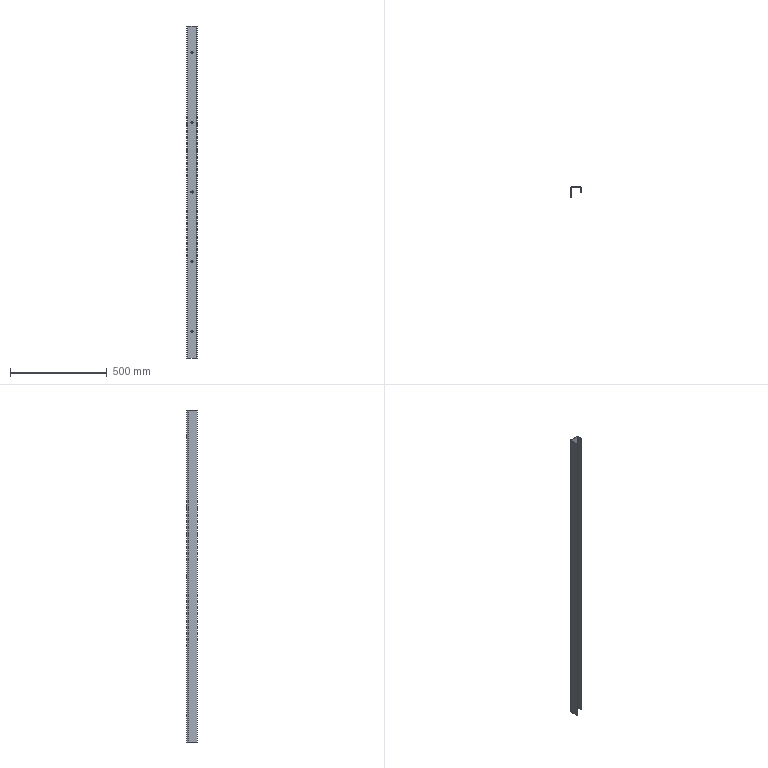Part | STEP file | SYL_0392D6J1SYL0380DJ10-1409429 | 1 solid | 32 faces | box 55 x 53 x 1714 mm | volume 657582 mm3 | plane 18 | cylinder 14 | commonest cylinder face diameters 10.5 x10 6 x2 12 x2
STEP:
#1=CARTESIAN_POINT('',(27.5,-3.,-725.25));
#2=VERTEX_POINT('',#1);
#3=CARTESIAN_POINT('',(27.5,0.,-725.25));
#4=VERTEX_POINT('',#3);
#5=CARTESIAN_POINT('',(27.5,0.,-725.25));
#6=DIRECTION('',(0.,1.,0.));
#7=VECTOR('',#6,1000.);
#8=LINE('',#5,#7);
#9=EDGE_CURVE('',#2,#4,#8,.T.);
#10=ORIENTED_EDGE('',*,*,#9,.F.);
#11=CARTESIAN_POINT('',(27.5,-3.,-714.75));
#12=VERTEX_POINT('',#11);
#13=CARTESIAN_POINT('',(27.5,-3.,-720.));
#14=DIRECTION('',(0.,-1.,0.));
#15=DIRECTION('',(0.,0.,-1.));
#16=AXIS2_PLACEMENT_3D('',#13,#14,#15);
#17=CIRCLE('',#16,5.25);
#18=EDGE_CURVE('',#2,#12,#17,.T.);
#19=ORIENTED_EDGE('',*,*,#18,.T.);
#20=CARTESIAN_POINT('',(27.5,0.,-714.75));
#21=VERTEX_POINT('',#20);
#22=CARTESIAN_POINT('',(27.5,0.,-714.75));
#23=DIRECTION('',(0.,1.,0.));
#24=VECTOR('',#23,1000.);
#25=LINE('',#22,#24);
#26=EDGE_CURVE('',#12,#21,#25,.T.);
#27=ORIENTED_EDGE('',*,*,#26,.T.);
#28=CARTESIAN_POINT('',(27.5,0.,-720.));
#29=DIRECTION('',(0.,-1.,0.));
#30=DIRECTION('',(0.,0.,-1.));
#31=AXIS2_PLACEMENT_3D('',#28,#29,#30);
#32=CIRCLE('',#31,5.25);
#33=EDGE_CURVE('',#4,#21,#32,.T.);
#34=ORIENTED_EDGE('',*,*,#33,.F.);
#35=EDGE_LOOP('',(#10,#19,#27,#34));
#36=FACE_OUTER_BOUND('',#35,.T.);
#37=CARTESIAN_POINT('',(27.5,0.,-720.));
#38=DIRECTION('',(0.,1.,0.));
#39=DIRECTION('',(0.,0.,1.));
#40=AXIS2_PLACEMENT_3D('',#37,#38,#39);
#41=CYLINDRICAL_SURFACE('',#40,5.25);
#42=ADVANCED_FACE('',(#36),#41,.F.);
#43=CARTESIAN_POINT('',(27.5,-3.,-365.25));
#44=VERTEX_POINT('',#43);
#45=CARTESIAN_POINT('',(27.5,0.,-365.25));
#46=VERTEX_POINT('',#45);
#47=CARTESIAN_POINT('',(27.5,0.,-365.25));
#48=DIRECTION('',(0.,1.,0.));
#49=VECTOR('',#48,1000.);
#50=LINE('',#47,#49);
#51=EDGE_CURVE('',#44,#46,#50,.T.);
#52=ORIENTED_EDGE('',*,*,#51,.F.);
#53=CARTESIAN_POINT('',(27.5,-3.,-354.75));
#54=VERTEX_POINT('',#53);
#55=CARTESIAN_POINT('',(27.5,-3.,-360.));
#56=DIRECTION('',(0.,-1.,0.));
#57=DIRECTION('',(0.,0.,-1.));
#58=AXIS2_PLACEMENT_3D('',#55,#56,#57);
#59=CIRCLE('',#58,5.25);
#60=EDGE_CURVE('',#44,#54,#59,.T.);
#61=ORIENTED_EDGE('',*,*,#60,.T.);
#62=CARTESIAN_POINT('',(27.5,0.,-354.75));
#63=VERTEX_POINT('',#62);
#64=CARTESIAN_POINT('',(27.5,0.,-354.75));
#65=DIRECTION('',(0.,1.,0.));
#66=VECTOR('',#65,1000.);
#67=LINE('',#64,#66);
#68=EDGE_CURVE('',#54,#63,#67,.T.);
#69=ORIENTED_EDGE('',*,*,#68,.T.);
#70=CARTESIAN_POINT('',(27.5,0.,-360.));
#71=DIRECTION('',(0.,-1.,0.));
#72=DIRECTION('',(0.,0.,-1.));
#73=AXIS2_PLACEMENT_3D('',#70,#71,#72);
#74=CIRCLE('',#73,5.25);
#75=EDGE_CURVE('',#46,#63,#74,.T.);
#76=ORIENTED_EDGE('',*,*,#75,.F.);
#77=EDGE_LOOP('',(#52,#61,#69,#76));
#78=FACE_OUTER_BOUND('',#77,.T.);
#79=CARTESIAN_POINT('',(27.5,0.,-360.));
#80=DIRECTION('',(0.,1.,0.));
#81=DIRECTION('',(0.,0.,1.));
#82=AXIS2_PLACEMENT_3D('',#79,#80,#81);
#83=CYLINDRICAL_SURFACE('',#82,5.25);
#84=ADVANCED_FACE('',(#78),#83,.F.);
#85=CARTESIAN_POINT('',(27.5,-3.,-5.25));
#86=VERTEX_POINT('',#85);
#87=CARTESIAN_POINT('',(27.5,0.,-5.25));
#88=VERTEX_POINT('',#87);
#89=CARTESIAN_POINT('',(27.5,0.,-5.25));
#90=DIRECTION('',(0.,1.,0.));
#91=VECTOR('',#90,1000.);
#92=LINE('',#89,#91);
#93=EDGE_CURVE('',#86,#88,#92,.T.);
#94=ORIENTED_EDGE('',*,*,#93,.F.);
#95=CARTESIAN_POINT('',(27.5,-3.,5.25));
#96=VERTEX_POINT('',#95);
#97=CARTESIAN_POINT('',(27.5,-3.,0.));
#98=DIRECTION('',(0.,-1.,0.));
#99=DIRECTION('',(0.,0.,-1.));
#100=AXIS2_PLACEMENT_3D('',#97,#98,#99);
#101=CIRCLE('',#100,5.25);
#102=EDGE_CURVE('',#86,#96,#101,.T.);
#103=ORIENTED_EDGE('',*,*,#102,.T.);
#104=CARTESIAN_POINT('',(27.5,0.,5.25));
#105=VERTEX_POINT('',#104);
#106=CARTESIAN_POINT('',(27.5,0.,5.25));
#107=DIRECTION('',(0.,1.,0.));
#108=VECTOR('',#107,1000.);
#109=LINE('',#106,#108);
#110=EDGE_CURVE('',#96,#105,#109,.T.);
#111=ORIENTED_EDGE('',*,*,#110,.T.);
#112=CARTESIAN_POINT('',(27.5,0.,0.));
#113=DIRECTION('',(0.,-1.,0.));
#114=DIRECTION('',(0.,0.,-1.));
#115=AXIS2_PLACEMENT_3D('',#112,#113,#114);
#116=CIRCLE('',#115,5.25);
#117=EDGE_CURVE('',#88,#105,#116,.T.);
#118=ORIENTED_EDGE('',*,*,#117,.F.);
#119=EDGE_LOOP('',(#94,#103,#111,#118));
#120=FACE_OUTER_BOUND('',#119,.T.);
#121=CARTESIAN_POINT('',(27.5,0.,0.));
#122=DIRECTION('',(0.,1.,0.));
#123=DIRECTION('',(0.,0.,1.));
#124=AXIS2_PLACEMENT_3D('',#121,#122,#123);
#125=CYLINDRICAL_SURFACE('',#124,5.25);
#126=ADVANCED_FACE('',(#120),#125,.F.);
#127=CARTESIAN_POINT('',(27.5,-3.,354.75));
#128=VERTEX_POINT('',#127);
#129=CARTESIAN_POINT('',(27.5,0.,354.75));
#130=VERTEX_POINT('',#129);
#131=CARTESIAN_POINT('',(27.5,0.,354.75));
#132=DIRECTION('',(0.,1.,0.));
#133=VECTOR('',#132,1000.);
#134=LINE('',#131,#133);
#135=EDGE_CURVE('',#128,#130,#134,.T.);
#136=ORIENTED_EDGE('',*,*,#135,.F.);
#137=CARTESIAN_POINT('',(27.5,-3.,365.25));
#138=VERTEX_POINT('',#137);
#139=CARTESIAN_POINT('',(27.5,-3.,360.));
#140=DIRECTION('',(0.,-1.,0.));
#141=DIRECTION('',(0.,0.,-1.));
#142=AXIS2_PLACEMENT_3D('',#139,#140,#141);
#143=CIRCLE('',#142,5.25);
#144=EDGE_CURVE('',#128,#138,#143,.T.);
#145=ORIENTED_EDGE('',*,*,#144,.T.);
#146=CARTESIAN_POINT('',(27.5,0.,365.25));
#147=VERTEX_POINT('',#146);
#148=CARTESIAN_POINT('',(27.5,0.,365.25));
#149=DIRECTION('',(0.,1.,0.));
#150=VECTOR('',#149,1000.);
#151=LINE('',#148,#150);
#152=EDGE_CURVE('',#138,#147,#151,.T.);
#153=ORIENTED_EDGE('',*,*,#152,.T.);
#154=CARTESIAN_POINT('',(27.5,0.,360.));
#155=DIRECTION('',(0.,-1.,0.));
#156=DIRECTION('',(0.,0.,-1.));
#157=AXIS2_PLACEMENT_3D('',#154,#155,#156);
#158=CIRCLE('',#157,5.25);
#159=EDGE_CURVE('',#130,#147,#158,.T.);
#160=ORIENTED_EDGE('',*,*,#159,.F.);
#161=EDGE_LOOP('',(#136,#145,#153,#160));
#162=FACE_OUTER_BOUND('',#161,.T.);
#163=CARTESIAN_POINT('',(27.5,0.,360.));
#164=DIRECTION('',(0.,1.,0.));
#165=DIRECTION('',(0.,0.,1.));
#166=AXIS2_PLACEMENT_3D('',#163,#164,#165);
#167=CYLINDRICAL_SURFACE('',#166,5.25);
#168=ADVANCED_FACE('',(#162),#167,.F.);
#169=CARTESIAN_POINT('',(27.5,-3.,714.75));
#170=VERTEX_POINT('',#169);
#171=CARTESIAN_POINT('',(27.5,0.,714.75));
#172=VERTEX_POINT('',#171);
#173=CARTESIAN_POINT('',(27.5,0.,714.75));
#174=DIRECTION('',(0.,1.,0.));
#175=VECTOR('',#174,1000.);
#176=LINE('',#173,#175);
#177=EDGE_CURVE('',#170,#172,#176,.T.);
#178=ORIENTED_EDGE('',*,*,#177,.F.);
#179=CARTESIAN_POINT('',(27.5,-3.,725.25));
#180=VERTEX_POINT('',#179);
#181=CARTESIAN_POINT('',(27.5,-3.,720.));
#182=DIRECTION('',(0.,-1.,0.));
#183=DIRECTION('',(0.,0.,-1.));
#184=AXIS2_PLACEMENT_3D('',#181,#182,#183);
#185=CIRCLE('',#184,5.25);
#186=EDGE_CURVE('',#170,#180,#185,.T.);
#187=ORIENTED_EDGE('',*,*,#186,.T.);
#188=CARTESIAN_POINT('',(27.5,0.,725.25));
#189=VERTEX_POINT('',#188);
#190=CARTESIAN_POINT('',(27.5,0.,725.25));
#191=DIRECTION('',(0.,1.,0.));
#192=VECTOR('',#191,1000.);
#193=LINE('',#190,#192);
#194=EDGE_CURVE('',#180,#189,#193,.T.);
#195=ORIENTED_EDGE('',*,*,#194,.T.);
#196=CARTESIAN_POINT('',(27.5,0.,720.));
#197=DIRECTION('',(0.,-1.,0.));
#198=DIRECTION('',(0.,0.,-1.));
#199=AXIS2_PLACEMENT_3D('',#196,#197,#198);
#200=CIRCLE('',#199,5.25);
#201=EDGE_CURVE('',#172,#189,#200,.T.);
#202=ORIENTED_EDGE('',*,*,#201,.F.);
#203=EDGE_LOOP('',(#178,#187,#195,#202));
#204=FACE_OUTER_BOUND('',#203,.T.);
#205=CARTESIAN_POINT('',(27.5,0.,720.));
#206=DIRECTION('',(0.,1.,0.));
#207=DIRECTION('',(0.,0.,1.));
#208=AXIS2_PLACEMENT_3D('',#205,#206,#207);
#209=CYLINDRICAL_SURFACE('',#208,5.25);
#210=ADVANCED_FACE('',(#204),#209,.F.);
#211=CARTESIAN_POINT('',(6.,-3.,-857.));
#212=VERTEX_POINT('',#211);
#213=CARTESIAN_POINT('',(6.,0.,-857.));
#214=VERTEX_POINT('',#213);
#215=CARTESIAN_POINT('',(6.,0.,-857.));
#216=DIRECTION('',(0.,1.,0.));
#217=VECTOR('',#216,1000.);
#218=LINE('',#215,#217);
#219=EDGE_CURVE('',#212,#214,#218,.T.);
#220=ORIENTED_EDGE('',*,*,#219,.F.);
#221=CARTESIAN_POINT('',(3.,-6.,-857.));
#222=VERTEX_POINT('',#221);
#223=CARTESIAN_POINT('',(6.,-6.,-857.));
#224=DIRECTION('',(0.,0.,-1.));
#225=DIRECTION('',(1.,0.,0.));
#226=AXIS2_PLACEMENT_3D('',#223,#224,#225);
#227=CIRCLE('',#226,3.);
#228=EDGE_CURVE('',#222,#212,#227,.T.);
#229=ORIENTED_EDGE('',*,*,#228,.F.);
#230=CARTESIAN_POINT('',(0.,-6.,-857.));
#231=VERTEX_POINT('',#230);
#232=CARTESIAN_POINT('',(0.,-6.,-857.));
#233=DIRECTION('',(-1.,0.,0.));
#234=VECTOR('',#233,1000.);
#235=LINE('',#232,#234);
#236=EDGE_CURVE('',#222,#231,#235,.T.);
#237=ORIENTED_EDGE('',*,*,#236,.T.);
#238=CARTESIAN_POINT('',(6.,-6.,-857.));
#239=DIRECTION('',(0.,0.,-1.));
#240=DIRECTION('',(-1.,0.,0.));
#241=AXIS2_PLACEMENT_3D('',#238,#239,#240);
#242=CIRCLE('',#241,6.);
#243=EDGE_CURVE('',#231,#214,#242,.T.);
#244=ORIENTED_EDGE('',*,*,#243,.T.);
#245=EDGE_LOOP('',(#220,#229,#237,#244));
#246=FACE_OUTER_BOUND('',#245,.T.);
#247=CARTESIAN_POINT('',(6.,-6.,-857.));
#248=DIRECTION('',(0.,0.,1.));
#249=DIRECTION('',(1.,0.,0.));
#250=AXIS2_PLACEMENT_3D('',#247,#248,#249);
#251=PLANE('',#250);
#252=ADVANCED_FACE('',(#246),#251,.F.);
#253=ORIENTED_EDGE('',*,*,#236,.F.);
#254=CARTESIAN_POINT('',(3.,-53.,-857.));
#255=VERTEX_POINT('',#254);
#256=CARTESIAN_POINT('',(3.,-6.,-857.));
#257=DIRECTION('',(0.,1.,0.));
#258=VECTOR('',#257,1000.);
#259=LINE('',#256,#258);
#260=EDGE_CURVE('',#255,#222,#259,.T.);
#261=ORIENTED_EDGE('',*,*,#260,.F.);
#262=CARTESIAN_POINT('',(0.,-53.,-857.));
#263=VERTEX_POINT('',#262);
#264=CARTESIAN_POINT('',(0.,-53.,-857.));
#265=DIRECTION('',(-1.,0.,0.));
#266=VECTOR('',#265,1000.);
#267=LINE('',#264,#266);
#268=EDGE_CURVE('',#255,#263,#267,.T.);
#269=ORIENTED_EDGE('',*,*,#268,.T.);
#270=CARTESIAN_POINT('',(0.,-53.,-857.));
#271=DIRECTION('',(0.,1.,0.));
#272=VECTOR('',#271,1000.);
#273=LINE('',#270,#272);
#274=EDGE_CURVE('',#263,#231,#273,.T.);
#275=ORIENTED_EDGE('',*,*,#274,.T.);
#276=EDGE_LOOP('',(#253,#261,#269,#275));
#277=FACE_OUTER_BOUND('',#276,.T.);
#278=CARTESIAN_POINT('',(0.,-53.,-857.));
#279=DIRECTION('',(0.,0.,1.));
#280=DIRECTION('',(0.,1.,0.));
#281=AXIS2_PLACEMENT_3D('',#278,#279,#280);
#282=PLANE('',#281);
#283=ADVANCED_FACE('',(#277),#282,.F.);
#284=ORIENTED_EDGE('',*,*,#268,.F.);
#285=CARTESIAN_POINT('',(3.,-53.,857.));
#286=VERTEX_POINT('',#285);
#287=CARTESIAN_POINT('',(3.,-53.,-857.));
#288=DIRECTION('',(0.,0.,-1.));
#289=VECTOR('',#288,1000.);
#290=LINE('',#287,#289);
#291=EDGE_CURVE('',#286,#255,#290,.T.);
#292=ORIENTED_EDGE('',*,*,#291,.F.);
#293=CARTESIAN_POINT('',(0.,-53.,857.));
#294=VERTEX_POINT('',#293);
#295=CARTESIAN_POINT('',(0.,-53.,857.));
#296=DIRECTION('',(-1.,0.,0.));
#297=VECTOR('',#296,1000.);
#298=LINE('',#295,#297);
#299=EDGE_CURVE('',#286,#294,#298,.T.);
#300=ORIENTED_EDGE('',*,*,#299,.T.);
#301=CARTESIAN_POINT('',(0.,-53.,857.));
#302=DIRECTION('',(0.,0.,-1.));
#303=VECTOR('',#302,1000.);
#304=LINE('',#301,#303);
#305=EDGE_CURVE('',#294,#263,#304,.T.);
#306=ORIENTED_EDGE('',*,*,#305,.T.);
#307=EDGE_LOOP('',(#284,#292,#300,#306));
#308=FACE_OUTER_BOUND('',#307,.T.);
#309=CARTESIAN_POINT('',(0.,-53.,857.));
#310=DIRECTION('',(0.,1.,0.));
#311=DIRECTION('',(0.,0.,-1.));
#312=AXIS2_PLACEMENT_3D('',#309,#310,#311);
#313=PLANE('',#312);
#314=ADVANCED_FACE('',(#308),#313,.F.);
#315=ORIENTED_EDGE('',*,*,#299,.F.);
#316=CARTESIAN_POINT('',(3.,-6.,857.));
#317=VERTEX_POINT('',#316);
#318=CARTESIAN_POINT('',(3.,-6.,857.));
#319=DIRECTION('',(0.,-1.,0.));
#320=VECTOR('',#319,1000.);
#321=LINE('',#318,#320);
#322=EDGE_CURVE('',#317,#286,#321,.T.);
#323=ORIENTED_EDGE('',*,*,#322,.F.);
#324=CARTESIAN_POINT('',(0.,-6.,857.));
#325=VERTEX_POINT('',#324);
#326=CARTESIAN_POINT('',(0.,-6.,857.));
#327=DIRECTION('',(-1.,0.,0.));
#328=VECTOR('',#327,1000.);
#329=LINE('',#326,#328);
#330=EDGE_CURVE('',#317,#325,#329,.T.);
#331=ORIENTED_EDGE('',*,*,#330,.T.);
#332=CARTESIAN_POINT('',(0.,-6.,857.));
#333=DIRECTION('',(0.,-1.,0.));
#334=VECTOR('',#333,1000.);
#335=LINE('',#332,#334);
#336=EDGE_CURVE('',#325,#294,#335,.T.);
#337=ORIENTED_EDGE('',*,*,#336,.T.);
#338=EDGE_LOOP('',(#315,#323,#331,#337));
#339=FACE_OUTER_BOUND('',#338,.T.);
#340=CARTESIAN_POINT('',(0.,-6.,857.));
#341=DIRECTION('',(0.,0.,-1.));
#342=DIRECTION('',(0.,-1.,0.));
#343=AXIS2_PLACEMENT_3D('',#340,#341,#342);
#344=PLANE('',#343);
#345=ADVANCED_FACE('',(#339),#344,.F.);
#346=ORIENTED_EDGE('',*,*,#330,.F.);
#347=CARTESIAN_POINT('',(6.,-3.,857.));
#348=VERTEX_POINT('',#347);
#349=CARTESIAN_POINT('',(6.,-6.,857.));
#350=DIRECTION('',(0.,0.,1.));
#351=DIRECTION('',(1.,0.,0.));
#352=AXIS2_PLACEMENT_3D('',#349,#350,#351);
#353=CIRCLE('',#352,3.);
#354=EDGE_CURVE('',#348,#317,#353,.T.);
#355=ORIENTED_EDGE('',*,*,#354,.F.);
#356=CARTESIAN_POINT('',(6.,0.,857.));
#357=VERTEX_POINT('',#356);
#358=CARTESIAN_POINT('',(6.,0.,857.));
#359=DIRECTION('',(0.,1.,0.));
#360=VECTOR('',#359,1000.);
#361=LINE('',#358,#360);
#362=EDGE_CURVE('',#348,#357,#361,.T.);
#363=ORIENTED_EDGE('',*,*,#362,.T.);
#364=CARTESIAN_POINT('',(6.,-6.,857.));
#365=DIRECTION('',(0.,0.,1.));
#366=DIRECTION('',(0.,1.,0.));
#367=AXIS2_PLACEMENT_3D('',#364,#365,#366);
#368=CIRCLE('',#367,6.);
#369=EDGE_CURVE('',#357,#325,#368,.T.);
#370=ORIENTED_EDGE('',*,*,#369,.T.);
#371=EDGE_LOOP('',(#346,#355,#363,#370));
#372=FACE_OUTER_BOUND('',#371,.T.);
#373=CARTESIAN_POINT('',(6.,-6.,857.));
#374=DIRECTION('',(0.,0.,-1.));
#375=DIRECTION('',(-1.,0.,0.));
#376=AXIS2_PLACEMENT_3D('',#373,#374,#375);
#377=PLANE('',#376);
#378=ADVANCED_FACE('',(#372),#377,.F.);
#379=ORIENTED_EDGE('',*,*,#362,.F.);
#380=CARTESIAN_POINT('',(49.,-3.,857.));
#381=VERTEX_POINT('',#380);
#382=CARTESIAN_POINT('',(49.,-3.,857.));
#383=DIRECTION('',(-1.,0.,0.));
#384=VECTOR('',#383,1000.);
#385=LINE('',#382,#384);
#386=EDGE_CURVE('',#381,#348,#385,.T.);
#387=ORIENTED_EDGE('',*,*,#386,.F.);
#388=CARTESIAN_POINT('',(49.,0.,857.));
#389=VERTEX_POINT('',#388);
#390=CARTESIAN_POINT('',(49.,0.,857.));
#391=DIRECTION('',(0.,1.,0.));
#392=VECTOR('',#391,1000.);
#393=LINE('',#390,#392);
#394=EDGE_CURVE('',#381,#389,#393,.T.);
#395=ORIENTED_EDGE('',*,*,#394,.T.);
#396=CARTESIAN_POINT('',(49.,0.,857.));
#397=DIRECTION('',(-1.,0.,0.));
#398=VECTOR('',#397,1000.);
#399=LINE('',#396,#398);
#400=EDGE_CURVE('',#389,#357,#399,.T.);
#401=ORIENTED_EDGE('',*,*,#400,.T.);
#402=EDGE_LOOP('',(#379,#387,#395,#401));
#403=FACE_OUTER_BOUND('',#402,.T.);
#404=CARTESIAN_POINT('',(49.,0.,857.));
#405=DIRECTION('',(0.,0.,-1.));
#406=DIRECTION('',(-1.,0.,0.));
#407=AXIS2_PLACEMENT_3D('',#404,#405,#406);
#408=PLANE('',#407);
#409=ADVANCED_FACE('',(#403),#408,.F.);
#410=ORIENTED_EDGE('',*,*,#394,.F.);
#411=CARTESIAN_POINT('',(52.,-6.,857.));
#412=VERTEX_POINT('',#411);
#413=CARTESIAN_POINT('',(49.,-6.,857.));
#414=DIRECTION('',(0.,0.,1.));
#415=DIRECTION('',(1.,0.,0.));
#416=AXIS2_PLACEMENT_3D('',#413,#414,#415);
#417=CIRCLE('',#416,3.);
#418=EDGE_CURVE('',#412,#381,#417,.T.);
#419=ORIENTED_EDGE('',*,*,#418,.F.);
#420=CARTESIAN_POINT('',(55.,-6.,857.));
#421=VERTEX_POINT('',#420);
#422=CARTESIAN_POINT('',(55.,-6.,857.));
#423=DIRECTION('',(1.,0.,0.));
#424=VECTOR('',#423,1000.);
#425=LINE('',#422,#424);
#426=EDGE_CURVE('',#412,#421,#425,.T.);
#427=ORIENTED_EDGE('',*,*,#426,.T.);
#428=CARTESIAN_POINT('',(49.,-6.,857.));
#429=DIRECTION('',(0.,0.,1.));
#430=DIRECTION('',(1.,0.,0.));
#431=AXIS2_PLACEMENT_3D('',#428,#429,#430);
#432=CIRCLE('',#431,6.);
#433=EDGE_CURVE('',#421,#389,#432,.T.);
#434=ORIENTED_EDGE('',*,*,#433,.T.);
#435=EDGE_LOOP('',(#410,#419,#427,#434));
#436=FACE_OUTER_BOUND('',#435,.T.);
#437=CARTESIAN_POINT('',(49.,-6.,857.));
#438=DIRECTION('',(0.,0.,-1.));
#439=DIRECTION('',(-1.,0.,0.));
#440=AXIS2_PLACEMENT_3D('',#437,#438,#439);
#441=PLANE('',#440);
#442=ADVANCED_FACE('',(#436),#441,.F.);
#443=ORIENTED_EDGE('',*,*,#426,.F.);
#444=CARTESIAN_POINT('',(52.,-30.,857.));
#445=VERTEX_POINT('',#444);
#446=CARTESIAN_POINT('',(52.,-30.,857.));
#447=DIRECTION('',(0.,1.,0.));
#448=VECTOR('',#447,1000.);
#449=LINE('',#446,#448);
#450=EDGE_CURVE('',#445,#412,#449,.T.);
#451=ORIENTED_EDGE('',*,*,#450,.F.);
#452=CARTESIAN_POINT('',(55.,-30.,857.));
#453=VERTEX_POINT('',#452);
#454=CARTESIAN_POINT('',(55.,-30.,857.));
#455=DIRECTION('',(1.,0.,0.));
#456=VECTOR('',#455,1000.);
#457=LINE('',#454,#456);
#458=EDGE_CURVE('',#445,#453,#457,.T.);
#459=ORIENTED_EDGE('',*,*,#458,.T.);
#460=CARTESIAN_POINT('',(55.,-30.,857.));
#461=DIRECTION('',(0.,1.,0.));
#462=VECTOR('',#461,1000.);
#463=LINE('',#460,#462);
#464=EDGE_CURVE('',#453,#421,#463,.T.);
#465=ORIENTED_EDGE('',*,*,#464,.T.);
#466=EDGE_LOOP('',(#443,#451,#459,#465));
#467=FACE_OUTER_BOUND('',#466,.T.);
#468=CARTESIAN_POINT('',(55.,-30.,857.));
#469=DIRECTION('',(0.,0.,-1.));
#470=DIRECTION('',(0.,1.,0.));
#471=AXIS2_PLACEMENT_3D('',#468,#469,#470);
#472=PLANE('',#471);
#473=ADVANCED_FACE('',(#467),#472,.F.);
#474=ORIENTED_EDGE('',*,*,#458,.F.);
#475=CARTESIAN_POINT('',(52.,-30.,-857.));
#476=VERTEX_POINT('',#475);
#477=CARTESIAN_POINT('',(52.,-30.,-857.));
#478=DIRECTION('',(0.,0.,1.));
#479=VECTOR('',#478,1000.);
#480=LINE('',#477,#479);
#481=EDGE_CURVE('',#476,#445,#480,.T.);
#482=ORIENTED_EDGE('',*,*,#481,.F.);
#483=CARTESIAN_POINT('',(55.,-30.,-857.));
#484=VERTEX_POINT('',#483);
#485=CARTESIAN_POINT('',(55.,-30.,-857.));
#486=DIRECTION('',(1.,0.,0.));
#487=VECTOR('',#486,1000.);
#488=LINE('',#485,#487);
#489=EDGE_CURVE('',#476,#484,#488,.T.);
#490=ORIENTED_EDGE('',*,*,#489,.T.);
#491=CARTESIAN_POINT('',(55.,-30.,-857.));
#492=DIRECTION('',(0.,0.,1.));
#493=VECTOR('',#492,1000.);
#494=LINE('',#491,#493);
#495=EDGE_CURVE('',#484,#453,#494,.T.);
#496=ORIENTED_EDGE('',*,*,#495,.T.);
#497=EDGE_LOOP('',(#474,#482,#490,#496));
#498=FACE_OUTER_BOUND('',#497,.T.);
#499=CARTESIAN_POINT('',(55.,-30.,-857.));
#500=DIRECTION('',(0.,1.,0.));
#501=DIRECTION('',(0.,0.,1.));
#502=AXIS2_PLACEMENT_3D('',#499,#500,#501);
#503=PLANE('',#502);
#504=ADVANCED_FACE('',(#498),#503,.F.);
#505=ORIENTED_EDGE('',*,*,#489,.F.);
#506=CARTESIAN_POINT('',(52.,-6.,-857.));
#507=VERTEX_POINT('',#506);
#508=CARTESIAN_POINT('',(52.,-30.,-857.));
#509=DIRECTION('',(0.,-1.,0.));
#510=VECTOR('',#509,1000.);
#511=LINE('',#508,#510);
#512=EDGE_CURVE('',#507,#476,#511,.T.);
#513=ORIENTED_EDGE('',*,*,#512,.F.);
#514=CARTESIAN_POINT('',(55.,-6.,-857.));
#515=VERTEX_POINT('',#514);
#516=CARTESIAN_POINT('',(55.,-6.,-857.));
#517=DIRECTION('',(1.,0.,0.));
#518=VECTOR('',#517,1000.);
#519=LINE('',#516,#518);
#520=EDGE_CURVE('',#507,#515,#519,.T.);
#521=ORIENTED_EDGE('',*,*,#520,.T.);
#522=CARTESIAN_POINT('',(55.,-6.,-857.));
#523=DIRECTION('',(0.,-1.,0.));
#524=VECTOR('',#523,1000.);
#525=LINE('',#522,#524);
#526=EDGE_CURVE('',#515,#484,#525,.T.);
#527=ORIENTED_EDGE('',*,*,#526,.T.);
#528=EDGE_LOOP('',(#505,#513,#521,#527));
#529=FACE_OUTER_BOUND('',#528,.T.);
#530=CARTESIAN_POINT('',(55.,-6.,-857.));
#531=DIRECTION('',(0.,0.,1.));
#532=DIRECTION('',(0.,-1.,0.));
#533=AXIS2_PLACEMENT_3D('',#530,#531,#532);
#534=PLANE('',#533);
#535=ADVANCED_FACE('',(#529),#534,.F.);
#536=ORIENTED_EDGE('',*,*,#520,.F.);
#537=CARTESIAN_POINT('',(49.,-3.,-857.));
#538=VERTEX_POINT('',#537);
#539=CARTESIAN_POINT('',(49.,-6.,-857.));
#540=DIRECTION('',(0.,0.,-1.));
#541=DIRECTION('',(1.,0.,0.));
#542=AXIS2_PLACEMENT_3D('',#539,#540,#541);
#543=CIRCLE('',#542,3.);
#544=EDGE_CURVE('',#538,#507,#543,.T.);
#545=ORIENTED_EDGE('',*,*,#544,.F.);
#546=CARTESIAN_POINT('',(49.,0.,-857.));
#547=VERTEX_POINT('',#546);
#548=CARTESIAN_POINT('',(49.,0.,-857.));
#549=DIRECTION('',(0.,1.,0.));
#550=VECTOR('',#549,1000.);
#551=LINE('',#548,#550);
#552=EDGE_CURVE('',#538,#547,#551,.T.);
#553=ORIENTED_EDGE('',*,*,#552,.T.);
#554=CARTESIAN_POINT('',(49.,-6.,-857.));
#555=DIRECTION('',(0.,0.,-1.));
#556=DIRECTION('',(0.,1.,0.));
#557=AXIS2_PLACEMENT_3D('',#554,#555,#556);
#558=CIRCLE('',#557,6.);
#559=EDGE_CURVE('',#547,#515,#558,.T.);
#560=ORIENTED_EDGE('',*,*,#559,.T.);
#561=EDGE_LOOP('',(#536,#545,#553,#560));
#562=FACE_OUTER_BOUND('',#561,.T.);
#563=CARTESIAN_POINT('',(49.,-6.,-857.));
#564=DIRECTION('',(0.,0.,1.));
#565=DIRECTION('',(1.,0.,0.));
#566=AXIS2_PLACEMENT_3D('',#563,#564,#565);
#567=PLANE('',#566);
#568=ADVANCED_FACE('',(#562),#567,.F.);
#569=CARTESIAN_POINT('',(27.5,-3.,720.));
#570=DIRECTION('',(0.,-1.,0.));
#571=DIRECTION('',(0.,0.,-1.));
#572=AXIS2_PLACEMENT_3D('',#569,#570,#571);
#573=CIRCLE('',#572,5.25);
#574=EDGE_CURVE('',#180,#170,#573,.T.);
#575=ORIENTED_EDGE('',*,*,#574,.T.);
#576=ORIENTED_EDGE('',*,*,#177,.T.);
#577=CARTESIAN_POINT('',(27.5,0.,720.));
#578=DIRECTION('',(0.,-1.,0.));
#579=DIRECTION('',(0.,0.,1.));
#580=AXIS2_PLACEMENT_3D('',#577,#578,#579);
#581=CIRCLE('',#580,5.25);
#582=EDGE_CURVE('',#189,#172,#581,.T.);
#583=ORIENTED_EDGE('',*,*,#582,.F.);
#584=ORIENTED_EDGE('',*,*,#194,.F.);
#585=EDGE_LOOP('',(#575,#576,#583,#584));
#586=FACE_OUTER_BOUND('',#585,.T.);
#587=CARTESIAN_POINT('',(27.5,0.,720.));
#588=DIRECTION('',(0.,1.,0.));
#589=DIRECTION('',(0.,0.,1.));
#590=AXIS2_PLACEMENT_3D('',#587,#588,#589);
#591=CYLINDRICAL_SURFACE('',#590,5.25);
#592=ADVANCED_FACE('',(#586),#591,.F.);
#593=CARTESIAN_POINT('',(27.5,-3.,360.));
#594=DIRECTION('',(0.,-1.,0.));
#595=DIRECTION('',(0.,0.,-1.));
#596=AXIS2_PLACEMENT_3D('',#593,#594,#595);
#597=CIRCLE('',#596,5.25);
#598=EDGE_CURVE('',#138,#128,#597,.T.);
#599=ORIENTED_EDGE('',*,*,#598,.T.);
#600=ORIENTED_EDGE('',*,*,#135,.T.);
#601=CARTESIAN_POINT('',(27.5,0.,360.));
#602=DIRECTION('',(0.,-1.,0.));
#603=DIRECTION('',(0.,0.,1.));
#604=AXIS2_PLACEMENT_3D('',#601,#602,#603);
#605=CIRCLE('',#604,5.25);
#606=EDGE_CURVE('',#147,#130,#605,.T.);
#607=ORIENTED_EDGE('',*,*,#606,.F.);
#608=ORIENTED_EDGE('',*,*,#152,.F.);
#609=EDGE_LOOP('',(#599,#600,#607,#608));
#610=FACE_OUTER_BOUND('',#609,.T.);
#611=CARTESIAN_POINT('',(27.5,0.,360.));
#612=DIRECTION('',(0.,1.,0.));
#613=DIRECTION('',(0.,0.,1.));
#614=AXIS2_PLACEMENT_3D('',#611,#612,#613);
#615=CYLINDRICAL_SURFACE('',#614,5.25);
#616=ADVANCED_FACE('',(#610),#615,.F.);
#617=CARTESIAN_POINT('',(27.5,-3.,0.));
#618=DIRECTION('',(0.,-1.,0.));
#619=DIRECTION('',(0.,0.,-1.));
#620=AXIS2_PLACEMENT_3D('',#617,#618,#619);
#621=CIRCLE('',#620,5.25);
#622=EDGE_CURVE('',#96,#86,#621,.T.);
#623=ORIENTED_EDGE('',*,*,#622,.T.);
#624=ORIENTED_EDGE('',*,*,#93,.T.);
#625=CARTESIAN_POINT('',(27.5,0.,0.));
#626=DIRECTION('',(0.,-1.,0.));
#627=DIRECTION('',(0.,0.,1.));
#628=AXIS2_PLACEMENT_3D('',#625,#626,#627);
#629=CIRCLE('',#628,5.25);
#630=EDGE_CURVE('',#105,#88,#629,.T.);
#631=ORIENTED_EDGE('',*,*,#630,.F.);
#632=ORIENTED_EDGE('',*,*,#110,.F.);
#633=EDGE_LOOP('',(#623,#624,#631,#632));
#634=FACE_OUTER_BOUND('',#633,.T.);
#635=CARTESIAN_POINT('',(27.5,0.,0.));
#636=DIRECTION('',(0.,1.,0.));
#637=DIRECTION('',(0.,0.,1.));
#638=AXIS2_PLACEMENT_3D('',#635,#636,#637);
#639=CYLINDRICAL_SURFACE('',#638,5.25);
#640=ADVANCED_FACE('',(#634),#639,.F.);
#641=CARTESIAN_POINT('',(27.5,-3.,-360.));
#642=DIRECTION('',(0.,-1.,0.));
#643=DIRECTION('',(0.,0.,-1.));
#644=AXIS2_PLACEMENT_3D('',#641,#642,#643);
#645=CIRCLE('',#644,5.25);
#646=EDGE_CURVE('',#54,#44,#645,.T.);
#647=ORIENTED_EDGE('',*,*,#646,.T.);
#648=ORIENTED_EDGE('',*,*,#51,.T.);
#649=CARTESIAN_POINT('',(27.5,0.,-360.));
#650=DIRECTION('',(0.,-1.,0.));
#651=DIRECTION('',(0.,0.,1.));
#652=AXIS2_PLACEMENT_3D('',#649,#650,#651);
#653=CIRCLE('',#652,5.25);
#654=EDGE_CURVE('',#63,#46,#653,.T.);
#655=ORIENTED_EDGE('',*,*,#654,.F.);
#656=ORIENTED_EDGE('',*,*,#68,.F.);
#657=EDGE_LOOP('',(#647,#648,#655,#656));
#658=FACE_OUTER_BOUND('',#657,.T.);
#659=CARTESIAN_POINT('',(27.5,0.,-360.));
#660=DIRECTION('',(0.,1.,0.));
#661=DIRECTION('',(0.,0.,1.));
#662=AXIS2_PLACEMENT_3D('',#659,#660,#661);
#663=CYLINDRICAL_SURFACE('',#662,5.25);
#664=ADVANCED_FACE('',(#658),#663,.F.);
#665=CARTESIAN_POINT('',(27.5,-3.,-720.));
#666=DIRECTION('',(0.,-1.,0.));
#667=DIRECTION('',(0.,0.,-1.));
#668=AXIS2_PLACEMENT_3D('',#665,#666,#667);
#669=CIRCLE('',#668,5.25);
#670=EDGE_CURVE('',#12,#2,#669,.T.);
#671=ORIENTED_EDGE('',*,*,#670,.T.);
#672=ORIENTED_EDGE('',*,*,#9,.T.);
#673=CARTESIAN_POINT('',(27.5,0.,-720.));
#674=DIRECTION('',(0.,-1.,0.));
#675=DIRECTION('',(0.,0.,1.));
#676=AXIS2_PLACEMENT_3D('',#673,#674,#675);
#677=CIRCLE('',#676,5.25);
#678=EDGE_CURVE('',#21,#4,#677,.T.);
#679=ORIENTED_EDGE('',*,*,#678,.F.);
#680=ORIENTED_EDGE('',*,*,#26,.F.);
#681=EDGE_LOOP('',(#671,#672,#679,#680));
#682=FACE_OUTER_BOUND('',#681,.T.);
#683=CARTESIAN_POINT('',(27.5,0.,-720.));
#684=DIRECTION('',(0.,1.,0.));
#685=DIRECTION('',(0.,0.,1.));
#686=AXIS2_PLACEMENT_3D('',#683,#684,#685);
#687=CYLINDRICAL_SURFACE('',#686,5.25);
#688=ADVANCED_FACE('',(#682),#687,.F.);
#689=CARTESIAN_POINT('',(49.,-3.,-857.));
#690=DIRECTION('',(1.,0.,0.));
#691=VECTOR('',#690,1000.);
#692=LINE('',#689,#691);
#693=EDGE_CURVE('',#212,#538,#692,.T.);
#694=ORIENTED_EDGE('',*,*,#693,.F.);
#695=ORIENTED_EDGE('',*,*,#219,.T.);
#696=CARTESIAN_POINT('',(6.,0.,-857.));
#697=DIRECTION('',(1.,0.,0.));
#698=VECTOR('',#697,1000.);
#699=LINE('',#696,#698);
#700=EDGE_CURVE('',#214,#547,#699,.T.);
#701=ORIENTED_EDGE('',*,*,#700,.T.);
#702=ORIENTED_EDGE('',*,*,#552,.F.);
#703=EDGE_LOOP('',(#694,#695,#701,#702));
#704=FACE_OUTER_BOUND('',#703,.T.);
#705=CARTESIAN_POINT('',(6.,0.,-857.));
#706=DIRECTION('',(0.,0.,1.));
#707=DIRECTION('',(1.,0.,0.));
#708=AXIS2_PLACEMENT_3D('',#705,#706,#707);
#709=PLANE('',#708);
#710=ADVANCED_FACE('',(#704),#709,.F.);
#711=ORIENTED_EDGE('',*,*,#559,.F.);
#712=CARTESIAN_POINT('',(49.,0.,-857.));
#713=DIRECTION('',(0.,0.,1.));
#714=VECTOR('',#713,1000.);
#715=LINE('',#712,#714);
#716=EDGE_CURVE('',#547,#389,#715,.T.);
#717=ORIENTED_EDGE('',*,*,#716,.T.);
#718=ORIENTED_EDGE('',*,*,#433,.F.);
#719=CARTESIAN_POINT('',(55.,-6.,857.));
#720=DIRECTION('',(0.,0.,-1.));
#721=VECTOR('',#720,1000.);
#722=LINE('',#719,#721);
#723=EDGE_CURVE('',#421,#515,#722,.T.);
#724=ORIENTED_EDGE('',*,*,#723,.T.);
#725=EDGE_LOOP('',(#711,#717,#718,#724));
#726=FACE_OUTER_BOUND('',#725,.T.);
#727=CARTESIAN_POINT('',(49.,-6.,-857.));
#728=DIRECTION('',(0.,0.,1.));
#729=DIRECTION('',(1.,0.,0.));
#730=AXIS2_PLACEMENT_3D('',#727,#728,#729);
#731=CYLINDRICAL_SURFACE('',#730,6.);
#732=ADVANCED_FACE('',(#726),#731,.T.);
#733=ORIENTED_EDGE('',*,*,#526,.F.);
#734=ORIENTED_EDGE('',*,*,#723,.F.);
#735=ORIENTED_EDGE('',*,*,#464,.F.);
#736=ORIENTED_EDGE('',*,*,#495,.F.);
#737=EDGE_LOOP('',(#733,#734,#735,#736));
#738=FACE_OUTER_BOUND('',#737,.T.);
#739=CARTESIAN_POINT('',(55.,-30.,-857.));
#740=DIRECTION('',(1.,0.,0.));
#741=DIRECTION('',(0.,1.,0.));
#742=AXIS2_PLACEMENT_3D('',#739,#740,#741);
#743=PLANE('',#742);
#744=ADVANCED_FACE('',(#738),#743,.T.);
#745=ORIENTED_EDGE('',*,*,#243,.F.);
#746=CARTESIAN_POINT('',(0.,-6.,-857.));
#747=DIRECTION('',(0.,0.,1.));
#748=VECTOR('',#747,1000.);
#749=LINE('',#746,#748);
#750=EDGE_CURVE('',#231,#325,#749,.T.);
#751=ORIENTED_EDGE('',*,*,#750,.T.);
#752=ORIENTED_EDGE('',*,*,#369,.F.);
#753=CARTESIAN_POINT('',(6.,0.,857.));
#754=DIRECTION('',(0.,0.,-1.));
#755=VECTOR('',#754,1000.);
#756=LINE('',#753,#755);
#757=EDGE_CURVE('',#357,#214,#756,.T.);
#758=ORIENTED_EDGE('',*,*,#757,.T.);
#759=EDGE_LOOP('',(#745,#751,#752,#758));
#760=FACE_OUTER_BOUND('',#759,.T.);
#761=CARTESIAN_POINT('',(6.,-6.,-857.));
#762=DIRECTION('',(0.,0.,1.));
#763=DIRECTION('',(1.,0.,0.));
#764=AXIS2_PLACEMENT_3D('',#761,#762,#763);
#765=CYLINDRICAL_SURFACE('',#764,6.);
#766=ADVANCED_FACE('',(#760),#765,.T.);
#767=ORIENTED_EDGE('',*,*,#201,.T.);
#768=ORIENTED_EDGE('',*,*,#582,.T.);
#769=EDGE_LOOP('',(#767,#768));
#770=FACE_BOUND('',#769,.T.);
#771=ORIENTED_EDGE('',*,*,#159,.T.);
#772=ORIENTED_EDGE('',*,*,#606,.T.);
#773=EDGE_LOOP('',(#771,#772));
#774=FACE_BOUND('',#773,.T.);
#775=ORIENTED_EDGE('',*,*,#117,.T.);
#776=ORIENTED_EDGE('',*,*,#630,.T.);
#777=EDGE_LOOP('',(#775,#776));
#778=FACE_BOUND('',#777,.T.);
#779=ORIENTED_EDGE('',*,*,#75,.T.);
#780=ORIENTED_EDGE('',*,*,#654,.T.);
#781=EDGE_LOOP('',(#779,#780));
#782=FACE_BOUND('',#781,.T.);
#783=ORIENTED_EDGE('',*,*,#33,.T.);
#784=ORIENTED_EDGE('',*,*,#678,.T.);
#785=EDGE_LOOP('',(#783,#784));
#786=FACE_BOUND('',#785,.T.);
#787=ORIENTED_EDGE('',*,*,#700,.F.);
#788=ORIENTED_EDGE('',*,*,#757,.F.);
#789=ORIENTED_EDGE('',*,*,#400,.F.);
#790=ORIENTED_EDGE('',*,*,#716,.F.);
#791=EDGE_LOOP('',(#787,#788,#789,#790));
#792=FACE_OUTER_BOUND('',#791,.T.);
#793=CARTESIAN_POINT('',(49.,0.,-857.));
#794=DIRECTION('',(0.,1.,0.));
#795=DIRECTION('',(1.,0.,0.));
#796=AXIS2_PLACEMENT_3D('',#793,#794,#795);
#797=PLANE('',#796);
#798=ADVANCED_FACE('',(#770,#774,#778,#782,#786,#792),#797,.T.);
#799=ORIENTED_EDGE('',*,*,#274,.F.);
#800=ORIENTED_EDGE('',*,*,#305,.F.);
#801=ORIENTED_EDGE('',*,*,#336,.F.);
#802=ORIENTED_EDGE('',*,*,#750,.F.);
#803=EDGE_LOOP('',(#799,#800,#801,#802));
#804=FACE_OUTER_BOUND('',#803,.T.);
#805=CARTESIAN_POINT('',(0.,-6.,-857.));
#806=DIRECTION('',(-1.,0.,0.));
#807=DIRECTION('',(0.,0.,1.));
#808=AXIS2_PLACEMENT_3D('',#805,#806,#807);
#809=PLANE('',#808);
#810=ADVANCED_FACE('',(#804),#809,.T.);
#811=ORIENTED_EDGE('',*,*,#544,.T.);
#812=CARTESIAN_POINT('',(52.,-6.,-857.));
#813=DIRECTION('',(0.,0.,-1.));
#814=VECTOR('',#813,1000.);
#815=LINE('',#812,#814);
#816=EDGE_CURVE('',#412,#507,#815,.T.);
#817=ORIENTED_EDGE('',*,*,#816,.F.);
#818=ORIENTED_EDGE('',*,*,#418,.T.);
#819=CARTESIAN_POINT('',(49.,-3.,-857.));
#820=DIRECTION('',(0.,0.,1.));
#821=VECTOR('',#820,1000.);
#822=LINE('',#819,#821);
#823=EDGE_CURVE('',#538,#381,#822,.T.);
#824=ORIENTED_EDGE('',*,*,#823,.F.);
#825=EDGE_LOOP('',(#811,#817,#818,#824));
#826=FACE_OUTER_BOUND('',#825,.T.);
#827=CARTESIAN_POINT('',(49.,-6.,-857.));
#828=DIRECTION('',(0.,0.,1.));
#829=DIRECTION('',(1.,0.,0.));
#830=AXIS2_PLACEMENT_3D('',#827,#828,#829);
#831=CYLINDRICAL_SURFACE('',#830,3.);
#832=ADVANCED_FACE('',(#826),#831,.F.);
#833=ORIENTED_EDGE('',*,*,#512,.T.);
#834=ORIENTED_EDGE('',*,*,#481,.T.);
#835=ORIENTED_EDGE('',*,*,#450,.T.);
#836=ORIENTED_EDGE('',*,*,#816,.T.);
#837=EDGE_LOOP('',(#833,#834,#835,#836));
#838=FACE_OUTER_BOUND('',#837,.T.);
#839=CARTESIAN_POINT('',(52.,-30.,-857.));
#840=DIRECTION('',(1.,0.,0.));
#841=DIRECTION('',(0.,1.,0.));
#842=AXIS2_PLACEMENT_3D('',#839,#840,#841);
#843=PLANE('',#842);
#844=ADVANCED_FACE('',(#838),#843,.F.);
#845=ORIENTED_EDGE('',*,*,#228,.T.);
#846=CARTESIAN_POINT('',(6.,-3.,-857.));
#847=DIRECTION('',(0.,0.,-1.));
#848=VECTOR('',#847,1000.);
#849=LINE('',#846,#848);
#850=EDGE_CURVE('',#348,#212,#849,.T.);
#851=ORIENTED_EDGE('',*,*,#850,.F.);
#852=ORIENTED_EDGE('',*,*,#354,.T.);
#853=CARTESIAN_POINT('',(3.,-6.,-857.));
#854=DIRECTION('',(0.,0.,1.));
#855=VECTOR('',#854,1000.);
#856=LINE('',#853,#855);
#857=EDGE_CURVE('',#222,#317,#856,.T.);
#858=ORIENTED_EDGE('',*,*,#857,.F.);
#859=EDGE_LOOP('',(#845,#851,#852,#858));
#860=FACE_OUTER_BOUND('',#859,.T.);
#861=CARTESIAN_POINT('',(6.,-6.,-857.));
#862=DIRECTION('',(0.,0.,1.));
#863=DIRECTION('',(1.,0.,0.));
#864=AXIS2_PLACEMENT_3D('',#861,#862,#863);
#865=CYLINDRICAL_SURFACE('',#864,3.);
#866=ADVANCED_FACE('',(#860),#865,.F.);
#867=ORIENTED_EDGE('',*,*,#186,.F.);
#868=ORIENTED_EDGE('',*,*,#574,.F.);
#869=EDGE_LOOP('',(#867,#868));
#870=FACE_BOUND('',#869,.T.);
#871=ORIENTED_EDGE('',*,*,#144,.F.);
#872=ORIENTED_EDGE('',*,*,#598,.F.);
#873=EDGE_LOOP('',(#871,#872));
#874=FACE_BOUND('',#873,.T.);
#875=ORIENTED_EDGE('',*,*,#102,.F.);
#876=ORIENTED_EDGE('',*,*,#622,.F.);
#877=EDGE_LOOP('',(#875,#876));
#878=FACE_BOUND('',#877,.T.);
#879=ORIENTED_EDGE('',*,*,#60,.F.);
#880=ORIENTED_EDGE('',*,*,#646,.F.);
#881=EDGE_LOOP('',(#879,#880));
#882=FACE_BOUND('',#881,.T.);
#883=ORIENTED_EDGE('',*,*,#18,.F.);
#884=ORIENTED_EDGE('',*,*,#670,.F.);
#885=EDGE_LOOP('',(#883,#884));
#886=FACE_BOUND('',#885,.T.);
#887=ORIENTED_EDGE('',*,*,#693,.T.);
#888=ORIENTED_EDGE('',*,*,#823,.T.);
#889=ORIENTED_EDGE('',*,*,#386,.T.);
#890=ORIENTED_EDGE('',*,*,#850,.T.);
#891=EDGE_LOOP('',(#887,#888,#889,#890));
#892=FACE_OUTER_BOUND('',#891,.T.);
#893=CARTESIAN_POINT('',(49.,-3.,-857.));
#894=DIRECTION('',(0.,1.,0.));
#895=DIRECTION('',(1.,0.,0.));
#896=AXIS2_PLACEMENT_3D('',#893,#894,#895);
#897=PLANE('',#896);
#898=ADVANCED_FACE('',(#870,#874,#878,#882,#886,#892),#897,.F.);
#899=ORIENTED_EDGE('',*,*,#260,.T.);
#900=ORIENTED_EDGE('',*,*,#857,.T.);
#901=ORIENTED_EDGE('',*,*,#322,.T.);
#902=ORIENTED_EDGE('',*,*,#291,.T.);
#903=EDGE_LOOP('',(#899,#900,#901,#902));
#904=FACE_OUTER_BOUND('',#903,.T.);
#905=CARTESIAN_POINT('',(3.,-6.,-857.));
#906=DIRECTION('',(-1.,0.,0.));
#907=DIRECTION('',(0.,0.,1.));
#908=AXIS2_PLACEMENT_3D('',#905,#906,#907);
#909=PLANE('',#908);
#910=ADVANCED_FACE('',(#904),#909,.F.);
#911=CLOSED_SHELL('',(#42,#84,#126,#168,#210,#252,#283,#314,#345,#378,#409,#442,#473,#504,#535,#568,#592,#616,#640,#664,#688,#710,#732,#744,#766,#798,#810,#832,#844,#866,#898,#910));
#912=MANIFOLD_SOLID_BREP('',#911);
#913=CARTESIAN_POINT('',(0.,0.,0.));
#914=DIRECTION('',(0.,0.,1.));
#915=DIRECTION('',(1.,0.,0.));
#916=AXIS2_PLACEMENT_3D('',#913,#914,#915);
#917=(LENGTH_UNIT()NAMED_UNIT(*)SI_UNIT(.MILLI.,.METRE.));
#918=UNCERTAINTY_MEASURE_WITH_UNIT(LENGTH_MEASURE(0.00001),#917,'','');
#919=(NAMED_UNIT(*)PLANE_ANGLE_UNIT()SI_UNIT($,.RADIAN.));
#920=(NAMED_UNIT(*)SI_UNIT($,.STERADIAN.)SOLID_ANGLE_UNIT());
#921=(GEOMETRIC_REPRESENTATION_CONTEXT(3)GLOBAL_UNCERTAINTY_ASSIGNED_CONTEXT((#918))GLOBAL_UNIT_ASSIGNED_CONTEXT((#917,#919,#920))REPRESENTATION_CONTEXT('',''));
#922=ADVANCED_BREP_SHAPE_REPRESENTATION('',(#912,#916),#921);